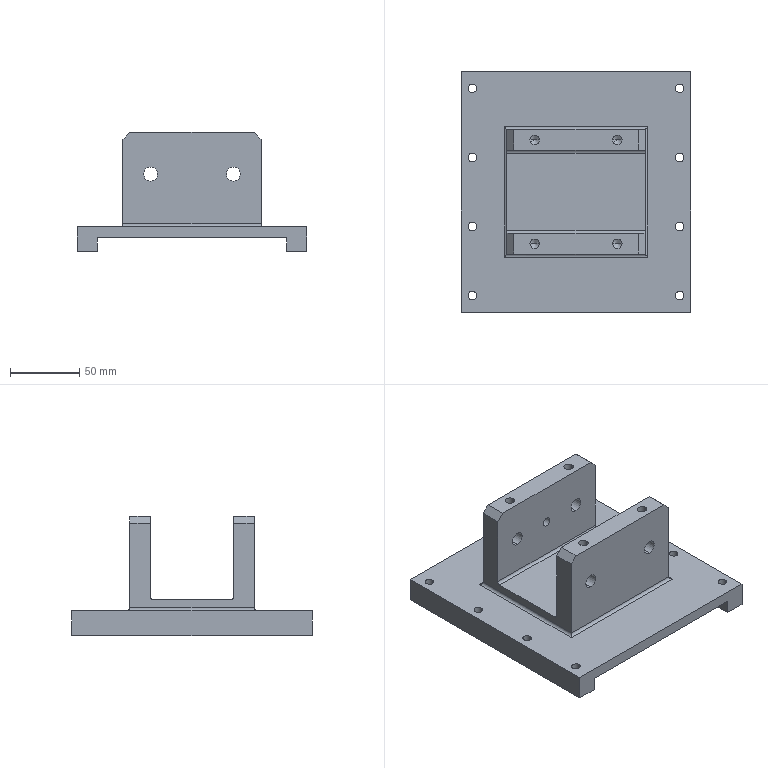NC program | NX | posted with a generic post | part box 166 x 174 x 86.2 mm
Whole program:
N10 G17 G21 G94 G90
(DRILLING_2 , TOOL : 倒角D10-90度)
N12 T03 M6
N14 G54
N16 G17 G0 G90 X-30. Y30.1 B0. C0. S1200 M3
N18 G43 Z20. H3
N20 G94 G81 G98 Z-4.1 B-180. F200. R3.
N22 X0.
N24 X30.
N26 G80
N28 G0 X30. Y30.1 Z20.
N30 M5
(DRILLING_2_COPY , TOOL : 钻头D6.8-73-105)
N32 T04 M6
N34 G54
N36 G17 G0 G90 X0. Y30.1 B0. C0. S1200 M3
N38 G43 Z20. H4
N40 G94 G83 G98 Z-20. B-180. F200. Q2. R3.
N42 G80
N44 G0 X0. Y30.1 Z20.
N46 M5
(DRILLING_2_COPY_COPY , TOOL : 上排M8-28-D6.2-70)
N48 T05 M6
N50 G54
N52 G17 G0 G90 X0. Y30.1 B0. C0. S300 M3
N54 G43 Z20. H5
N56 G84 G94 G98 Z-5. B-180. F375. R3.
N58 G80
N60 G0 X0. Y30.1 Z20.
N62 M5
(DRILLING_2_COPY_1 , TOOL : 钻头D10.0-95-130)
N64 T08 M6
N66 G54
N68 G17 G0 G90 X-30. Y30.1 B0. C0. S1200 M3
N70 G43 Z20. H8
N72 G94 G83 G98 Z-20. B-180. F200. Q2. R3.
N74 X30.
N76 G80
N78 G0 X30. Y30.1 Z20.
N80 M5
N82 M2